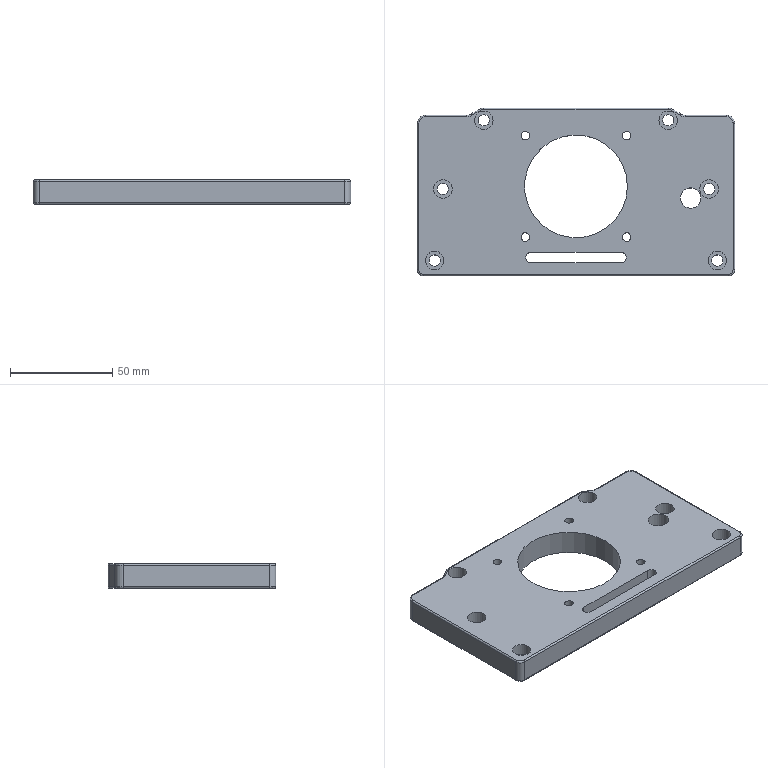Part | STEP file | 1 solid | 78 faces | box 155 x 82 x 12 mm | volume 118532 mm3 | cylinder 44 | plane 18 | spline 16 | commonest cylinder face diameters 1.5 x16 5.5 x6 8 x6 9 x6 4.2 x4 5 x2